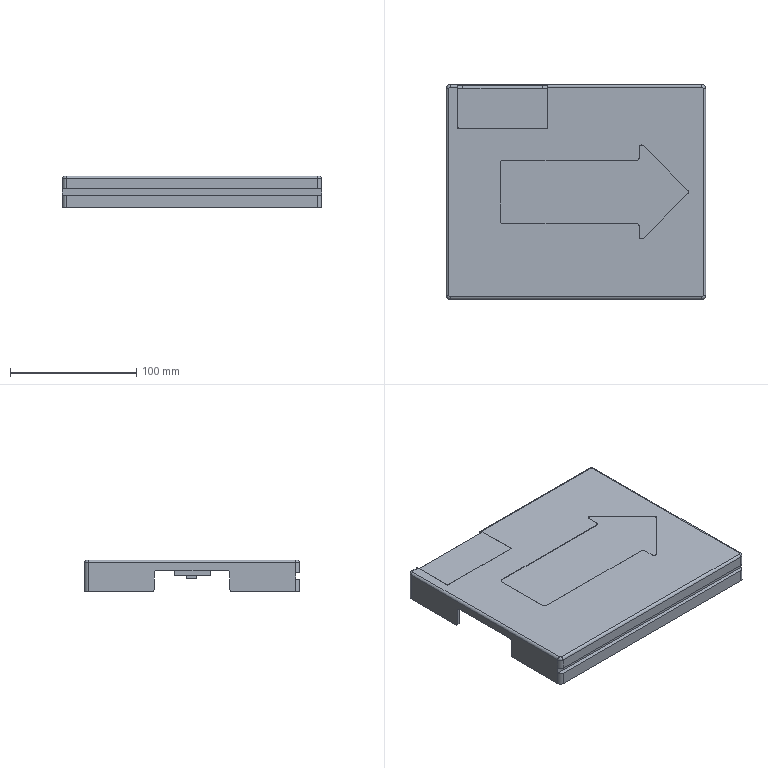NC program | NX | posted with a generic post | part box 205 x 170 x 25 mm
Lines 12675 to 13937 of 17262:
(ZLEVEL_PROFILE_1_COPY_1 , TOOL : D3R0.5)
N25306 T07 M6
N25308 G54
N25310 G17 G0 G90 X99.394 Y-30.534 B0. C0. S9500 M3
N25312 G43 Z30. H7
N25314 Z0.991
N25316 G94 G1 Z-0.009 F1000.
N25318 X99.711 Y-30.848
N25320 G3 X100.001 Y-30.925 R0.3
N25322 G1 X100.5 Y-30.789 F2500.
N25324 X102.5
N25326 X103.04 Y-30.943
N25328 X103.024 Y-30.869 Z-0.019
N25330 G3 X102.5 Y-30.709 R1.438
N25332 G1 X100.5
N25334 X99.999 Y-30.837
N25336 Y-30.78 Z-0.025
N25338 Y-30.732 Z-0.03
N25340 X100.5 Y-30.613
N25342 X102.5
N25344 X103.001 Y-30.741
N25346 Y-30.69 Z-0.038
N25348 Y-30.671 Z-0.046
N25350 G3 X102.5 Y-30.541 R1.095
N25352 G1 X100.5
N25354 X99.981 Y-30.655
N25356 Y-30.603 Z-0.055
N25358 Y-30.541 Z-0.065
N25360 X100.5 Y-30.435
N25362 X102.5
N25364 G2 X103. Y-30.565 R1.064
N25366 G1 X102.999 Y-30.47 Z-0.086
N25368 X102.5 Y-30.348
N25370 X100.5
N25372 X99.997 Y-30.447
N25374 Y-30.42 Z-0.099
N25376 X99.996 Y-30.365 Z-0.112
N25378 X100.5 Y-30.259
N25380 X102.5
N25382 X102.999 Y-30.387
N25384 Y-30.328 Z-0.127
N25386 Y-30.291 Z-0.142
N25388 G3 X102.5 Y-30.17 R1.236
N25390 G1 X100.5
N25392 X99.996 Y-30.272
N25394 Y-30.24 Z-0.158
N25396 X99.997 Y-30.185 Z-0.175
N25398 X100.5 Y-30.082
N25400 X102.5
N25402 X102.999 Y-30.199
N25404 X103. Y-30.146 Z-0.193
N25406 X103.001 Y-30.104 Z-0.211
N25408 X102.5 Y-29.994
N25410 X100.5
N25412 X99.997 Y-30.093
N25414 X99.998 Y-30.058 Z-0.231
N25416 X99.999 Y-30.004 Z-0.251
N25418 X100.5 Y-29.908
N25420 X102.5
N25422 X103.001 Y-30.006
N25424 Y-29.968 Z-0.273
N25426 X103.002 Y-29.918 Z-0.295
N25428 X102.5 Y-29.822
N25430 X100.5
N25432 X99.998 Y-29.913
N25434 Y-29.883 Z-0.318
N25436 Y-29.824 Z-0.342
N25438 G2 X100.5 Y-29.738 R3.15
N25440 G1 X102.5
N25442 X102.552 Y-29.741
N25444 X103.002 Y-29.829
N25446 Y-29.792 Z-0.367
N25448 Y-29.738 Z-0.392
N25450 X102.5 Y-29.655
N25452 X100.5
N25454 X99.999 Y-29.736
N25456 Y-29.696 Z-0.419
N25458 Y-29.65 Z-0.446
N25460 X100.5 Y-29.574
N25462 X102.5
N25464 X103.003 Y-29.643
N25466 Y-29.61 Z-0.475
N25468 X103.002 Y-29.566 Z-0.504
N25470 X102.5 Y-29.495
N25472 X100.5
N25474 X99.999 Y-29.569
N25476 Y-29.533 Z-0.534
N25478 X100. Y-29.491 Z-0.564
N25480 X100.5 Y-29.418
N25482 X102.5
N25484 G2 X103. Y-29.496 R37.012
N25486 G1 Y-29.457 Z-0.596
N25488 Y-29.419 Z-0.628
N25490 X102.5 Y-29.343
N25492 X100.5
N25494 X100. Y-29.417
N25496 Y-29.378 Z-0.661
N25498 Y-29.339 Z-0.694
N25500 G3 X100.5 Y-29.271 R1996.585
N25502 G1 X102.5
N25504 X103. Y-29.338
N25506 Y-29.299 Z-0.729
N25508 Y-29.26 Z-0.764
N25510 X102.944
N25512 X102.5 Y-29.201
N25514 X100.5
N25516 G2 X100. Y-29.262 R13.454
N25518 G1 Y-29.228 Z-0.8
N25520 Y-29.201 Z-0.837
N25522 G3 X100.5 Y-29.134 R9.112
N25524 G1 X102.5
N25526 G3 X103. Y-29.199 R5.937
N25528 G1 Y-29.164 Z-0.874
N25530 Y-29.136 Z-0.912
N25532 G2 X102.5 Y-29.069 R5.444
N25534 G1 X100.5
N25536 G3 X100.103 Y-29.135 R1.782
N25538 G1 X100. Y-29.138
N25540 Y-29.101 Z-0.951
N25542 Y-29.073 Z-0.99
N25544 G3 X100.255 Y-29.031 R0.597
N25546 G1 X100.5 Y-29.008
N25548 X102.5
N25550 G2 X102.895 Y-29.069 R1.306
N25552 G1 X103. Y-29.07
N25554 Y-29.037 Z-1.03
N25556 X103.001 Y-29.001 Z-1.07
N25558 X102.5 Y-28.95
N25560 X100.5
N25562 X100.348 Y-28.96
N25564 G2 X100. Y-29.007 R1.243
N25566 G1 Y-28.975 Z-1.111
N25568 Y-28.948 Z-1.152
N25570 G3 X100.348 Y-28.903 R1.222
N25572 G1 X100.5 Y-28.894
N25574 X102.5
N25576 X103.001 Y-28.943
N25578 Y-28.921 Z-1.195
N25580 Y-28.893 Z-1.237
N25582 X102.5 Y-28.842
N25584 X100.5
N25586 X100.348 Y-28.854
N25588 G2 X100. Y-28.899 R1.238
N25590 G1 Y-28.873 Z-1.281
N25592 Y-28.853 Z-1.324
N25594 G3 X100.348 Y-28.803 R1.115
N25596 G1 X100.5 Y-28.794
N25598 X102.5
N25600 X103.001 Y-28.847
N25602 Y-28.826 Z-1.369
N25604 X103. Y-28.8 Z-1.413
N25606 X102.5 Y-28.749
N25608 X100.5
N25610 G3 X100.111 Y-28.799 R2.259
N25612 G1 X100.056 Y-28.817
N25614 X100. Y-28.805
N25616 Y-28.778 Z-1.458
N25618 Y-28.758 Z-1.504
N25620 X100.103 Y-28.755
N25622 G2 X100.5 Y-28.707 R3.348
N25624 G1 X102.5
N25626 G3 X103.001 Y-28.754 R4.196
N25628 G1 Y-28.738 Z-1.55
N25630 Y-28.714 Z-1.596
N25632 G2 X102.5 Y-28.669 R6.317
N25634 G1 X100.5
N25636 G3 X100.103 Y-28.715 R2.341
N25638 G1 X99.999 Y-28.718
N25640 Y-28.701 Z-1.643
N25642 Y-28.688 Z-1.69
N25644 X100.103 Y-28.686
N25646 G2 X100.5 Y-28.635 R1.961
N25648 G1 X102.5
N25650 X103.003 Y-28.683
N25652 Y-28.671 Z-1.737
N25654 Y-28.654 Z-1.785
N25656 X102.5 Y-28.604
N25658 X100.5
N25660 G3 X100.103 Y-28.656 R1.723
N25662 G1 X99.999 Y-28.659
N25664 Y-28.641 Z-1.833
N25666 Y-28.629 Z-1.881
N25668 X100.103 Y-28.626
N25670 G2 X100.5 Y-28.578 R2.479
N25672 G1 X102.5
N25674 X103.003 Y-28.624
N25676 Y-28.615 Z-1.93
N25678 Y-28.599 Z-1.978
N25680 X102.5 Y-28.555
N25682 X100.5
N25684 G3 X100.103 Y-28.6 R3.094
N25686 G1 X99.999 Y-28.602
N25688 X99.998 Y-28.589 Z-2.028
N25690 Y-28.585 Z-2.077
N25692 X100.103 Y-28.58
N25694 G2 X100.5 Y-28.536 R2.159
N25696 G1 X102.5
N25698 G2 X103.002 Y-28.583 R25.83
N25700 G1 Y-28.572 Z-2.126
N25702 X103.001 Y-28.568 Z-2.176
N25704 X102.5 Y-28.521
N25706 X100.5
N25708 X100.232 Y-28.546
N25710 G2 X99.999 Y-28.571 R0.934
N25712 G1 Y-28.564 Z-2.225
N25714 Y-28.56 Z-2.275
N25716 X100.16 Y-28.546
N25718 G2 X100.5 Y-28.51 R2.032
N25720 G1 X102.5
N25722 G3 X103. Y-28.553 R6.443
N25724 G1 Y-28.546 Z-2.325
N25726 Y-28.539 Z-2.375
N25728 G2 X102.5 Y-28.503 R5.294
N25730 G1 X100.5
N25732 G3 X100. Y-28.549 R57.724
N25734 G1 Y-28.54 Z-2.475
N25736 X100.5 Y-28.5
N25738 X102.5
N25740 G3 X103. Y-28.53 R3.832
N25742 G1 Y-28.529 Z-2.575
N25744 G2 X102.5 Y-28.5 R3.541
N25746 G1 X100.5
N25748 X100. Y-28.536
N25750 Y-28.534 Z-2.675
N25752 X100.5 Y-28.5
N25754 X100.616
N25756 X101.802
N25758 X101.863
N25760 X102.408
N25762 X102.5
N25764 G3 X103. Y-28.527 R3.401
N25766 G1 Y-28.525 Z-2.775
N25768 G2 X102.5 Y-28.5 R3.458
N25770 G1 X102.408
N25772 X101.863
N25774 X101.802
N25776 X101.756
N25778 X100.616
N25780 X100.5
N25782 X100. Y-28.532
N25784 Y-28.531 Z-2.875
N25786 G2 X100.5 Y-28.5 R8.281
N25788 G1 X100.616
N25790 X101.802
N25792 X101.863
N25794 X102.408
N25796 X102.5
N25798 G3 X103. Y-28.524 R3.678
N25800 G1 Y-28.522 Z-2.975
N25802 G2 X102.5 Y-28.5 R3.929
N25804 G1 X102.408
N25806 X101.863
N25808 X101.802
N25810 X101.756
N25812 X100.616
N25814 X100.5
N25816 G3 X100. Y-28.529 R7.641
N25818 G1 Y-28.527 Z-3.075
N25820 G2 X100.5 Y-28.5 R202.736
N25822 G1 X100.616
N25824 X101.802
N25826 X101.863
N25828 X102.408
N25830 X102.5
N25832 G3 X103. Y-28.521 R4.217
N25834 G1 Y-28.519 Z-3.175
N25836 G2 X102.5 Y-28.5 R4.551
N25838 G1 X102.408
N25840 X101.863
N25842 X101.802
N25844 X101.756
N25846 X100.616
N25848 X100.5
N25850 X100. Y-28.525
N25852 Y-28.523 Z-3.275
N25854 X100.5 Y-28.5
N25856 X100.616
N25858 X101.802
N25860 X101.863
N25862 X102.408
N25864 X102.5
N25866 G3 X103. Y-28.518 R4.942
N25868 G1 Y-28.516 Z-3.375
N25870 G2 X102.5 Y-28.5 R5.408
N25872 G1 X102.408
N25874 X101.863
N25876 X101.802
N25878 X101.756
N25880 X100.616
N25882 X100.5
N25884 X100. Y-28.522
N25886 Y-28.52 Z-3.475
N25888 X100.5 Y-28.5
N25890 X100.616
N25892 X101.802
N25894 X101.863
N25896 X102.408
N25898 X102.5
N25900 G3 X103. Y-28.515 R5.363
N25902 G1 Y-28.513 Z-3.575
N25904 G2 X102.5 Y-28.5 R5.209
N25906 G1 X102.408
N25908 X101.863
N25910 X101.802
N25912 X101.756
N25914 X100.616
N25916 X100.5
N25918 X100. Y-28.519
N25920 Y-28.518 Z-3.675
N25922 X100.5 Y-28.5
N25924 X100.616
N25926 X101.802
N25928 X101.863
N25930 X102.408
N25932 X102.5
N25934 G3 X103. Y-28.512 R5.064
N25936 G1 Y-28.511 Z-3.775
N25938 G2 X102.5 Y-28.5 R4.927
N25940 G1 X102.408
N25942 X101.863
N25944 X101.802
N25946 X101.756
N25948 X100.616
N25950 X100.5
N25952 X100. Y-28.517
N25954 Y-28.516 Z-3.875
N25956 X100.5 Y-28.5
N25958 X100.616
N25960 X101.802
N25962 X101.863
N25964 X102.408
N25966 X102.5
N25968 G3 X103. Y-28.51 R4.797
N25970 G1 Y-28.508 Z-3.975
N25972 G2 X102.5 Y-28.5 R4.674
N25974 G1 X102.408
N25976 X101.863
N25978 X101.802
N25980 X101.756
N25982 X100.616
N25984 X100.5
N25986 X100. Y-28.515
N25988 Y-28.514 Z-4.075
N25990 X100.5 Y-28.5
N25992 X100.616
N25994 X101.802
N25996 X101.863
N25998 X102.408
N26000 X102.5
N26002 G3 X103. Y-28.507 R4.558
N26004 G1 Y-28.506 Z-4.175
N26006 G2 X102.5 Y-28.5 R4.446
N26008 G1 X102.408
N26010 X101.863
N26012 X101.802
N26014 X101.756
N26016 X100.616
N26018 X100.5
N26020 X100. Y-28.512
N26022 Y-28.511 Z-4.275
N26024 X100.5 Y-28.5
N26026 X100.616
N26028 X101.802
N26030 X101.863
N26032 X102.408
N26034 X102.5
N26036 G3 X103. Y-28.505 R4.385
N26038 G1 Z-4.375
N26040 G2 X102.5 Y-28.5 R4.589
N26042 G1 X102.408
N26044 X101.863
N26046 X101.802
N26048 X101.756
N26050 X100.616
N26052 X100.5
N26054 X100. Y-28.51
N26056 Z-4.475
N26058 X100.5 Y-28.5
N26060 X100.616
N26062 X101.802
N26064 X101.863
N26066 X102.408
N26068 X102.5
N26070 G3 X103. Y-28.504 R4.812
N26072 G1 Z-4.575
N26074 G2 X102.5 Y-28.5 R20.562
N26076 G1 X102.408
N26078 X101.863
N26080 X101.802
N26082 X101.756
N26084 X100.616
N26086 X100.5
N26088 X100. Y-28.51
N26090 Y-28.509 Z-4.675
N26092 X100.5 Y-28.5
N26094 X100.616
N26096 X101.802
N26098 X101.863
N26100 X102.408
N26102 X102.5
N26104 G3 X103. Y-28.503 R21.332
N26106 G1 Z-4.775
N26108 G2 X102.5 Y-28.5 R22.858
N26110 G1 X102.408
N26112 X101.863
N26114 X101.802
N26116 X101.756
N26118 X100.616
N26120 X100.5
N26122 X100. Y-28.509
N26124 Y-28.508 Z-4.875
N26126 X100.5 Y-28.5
N26128 X100.616
N26130 X101.802
N26132 X101.863
N26134 X102.408
N26136 X102.5
N26138 G3 X103. Y-28.503 R25.34
N26140 G1 Z-4.975
N26142 X102.5 Y-28.5
N26144 X102.408
N26146 X101.863
N26148 X101.802
N26150 X101.756
N26152 X100.616
N26154 X100.5
N26156 X100. Y-28.508
N26158 Y-28.507 Z-5.075
N26160 X100.5 Y-28.5
N26162 X100.616
N26164 X101.802
N26166 X101.863
N26168 X102.408
N26170 X102.5
N26172 X103. Y-28.503
N26174 Z-5.175
N26176 X102.5 Y-28.5
N26178 X102.408
N26180 X101.863
N26182 X101.802
N26184 X101.756
N26186 X100.616
N26188 X100.5
N26190 X100. Y-28.507
N26192 Z-5.275
N26194 X100.5 Y-28.5
N26196 X100.616
N26198 X101.802
N26200 X101.863
N26202 X102.408
N26204 X102.5
N26206 X103. Y-28.502
N26208 Z-5.375
N26210 X102.5 Y-28.5
N26212 X102.408
N26214 X101.863
N26216 X101.802
N26218 X101.756
N26220 X100.616
N26222 X100.5
N26224 X100. Y-28.506
N26226 Z-5.475
N26228 X100.5 Y-28.5
N26230 X100.616
N26232 X101.802
N26234 X101.863
N26236 X102.408
N26238 X102.5
N26240 X103. Y-28.502
N26242 Z-5.575
N26244 X102.5 Y-28.5
N26246 X102.408
N26248 X101.863
N26250 X101.802
N26252 X101.756
N26254 X100.616
N26256 X100.5
N26258 X100. Y-28.505
N26260 Z-5.675
N26262 X100.5 Y-28.5
N26264 X100.616
N26266 X101.802
N26268 X101.863
N26270 X102.408
N26272 X102.5
N26274 X102.552
N26276 X103. Y-28.502
N26278 Z-5.775
N26280 X102.5 Y-28.5
N26282 X102.408
N26284 X101.863
N26286 X101.802
N26288 X101.756
N26290 X100.616
N26292 X100.5
N26294 X100. Y-28.505
N26296 X100.001 Y-28.504 Z-5.875
N26298 X100.5 Y-28.5
N26300 X100.616
N26302 X101.802
N26304 X101.863
N26306 X102.408
N26308 X102.5
N26310 X103. Y-28.502
N26312 Y-28.501 Z-5.975
N26314 X102.5 Y-28.5
N26316 X102.408
N26318 X101.863
N26320 X101.802
N26322 X101.756
N26324 X100.616
N26326 X100.5
N26328 X100.001 Y-28.504
N26330 Y-28.503 Z-6.075
N26332 X100.5 Y-28.5
N26334 X100.616
N26336 X101.802
N26338 X101.863
N26340 X102.408
N26342 X102.5
N26344 X103. Y-28.501
N26346 Z-6.175
N26348 X102.5 Y-28.5
N26350 X102.408
N26352 X101.863
N26354 X101.802
N26356 X101.756
N26358 X100.616
N26360 X100.5
N26362 X100.001 Y-28.503
N26364 Z-6.275
N26366 X100.5 Y-28.5
N26368 X100.616
N26370 X101.802
N26372 X101.863
N26374 X102.408
N26376 X102.5
N26378 X103. Y-28.501
N26380 Z-6.375
N26382 X102.5 Y-28.5
N26384 X102.408
N26386 X101.863
N26388 X101.802
N26390 X101.756
N26392 X100.616
N26394 X100.5
N26396 X100.001 Y-28.503
N26398 Z-6.475
N26400 X100.5 Y-28.5
N26402 X100.616
N26404 X101.802
N26406 X101.863
N26408 X102.408
N26410 X102.5
N26412 X103. Y-28.501
N26414 Z-6.575
N26416 X102.5 Y-28.5
N26418 X102.408
N26420 X101.863
N26422 X101.802
N26424 X101.756
N26426 X100.616
N26428 X100.5
N26430 X100.001 Y-28.503
N26432 Z-6.675
N26434 X100.5 Y-28.5
N26436 X100.616
N26438 X101.802
N26440 X101.863
N26442 X102.408
N26444 X102.5
N26446 X103. Y-28.501
N26448 Z-6.775
N26450 X102.5 Y-28.5
N26452 X102.408
N26454 X101.863
N26456 X101.802
N26458 X101.756
N26460 X100.616
N26462 X100.5
N26464 X100.001 Y-28.503
N26466 Z-6.875
N26468 X100.5 Y-28.5
N26470 X100.616
N26472 X101.802
N26474 X101.863
N26476 X102.408
N26478 X102.5
N26480 X103. Y-28.501
N26482 Z-6.975
N26484 X102.5 Y-28.5
N26486 X102.408
N26488 X101.863
N26490 X101.802
N26492 X101.756
N26494 X100.616
N26496 X100.5
N26498 X100.001 Y-28.503
N26500 Z-7.075
N26502 X100.5 Y-28.5
N26504 X100.616
N26506 X101.802
N26508 X101.863
N26510 X102.408
N26512 X102.5
N26514 X103. Y-28.501
N26516 Z-7.175
N26518 X102.5 Y-28.5
N26520 X102.408
N26522 X101.863
N26524 X101.802
N26526 X101.756
N26528 X100.616
N26530 X100.5
N26532 X100.001 Y-28.503
N26534 Z-7.275
N26536 X100.5 Y-28.5
N26538 X100.616
N26540 X101.802
N26542 X101.863
N26544 X102.408
N26546 X102.5
N26548 X103. Y-28.501
N26550 Z-7.375
N26552 X102.5 Y-28.5
N26554 X102.408
N26556 X101.863
N26558 X101.802
N26560 X101.756
N26562 X100.616
N26564 X100.5
N26566 X100.001 Y-28.503
N26568 Z-7.475
N26570 X100.5 Y-28.5
N26572 X100.616
N26574 X101.802
N26576 X101.863
N26578 X102.408
N26580 X102.5
N26582 X103. Y-28.501
N26584 Z-7.575
N26586 X102.5 Y-28.5
N26588 X102.408
N26590 X101.863
N26592 X101.802
N26594 X101.756
N26596 X100.616
N26598 X100.5
N26600 X100.001 Y-28.503
N26602 Z-7.675
N26604 X100.5 Y-28.5
N26606 X100.616
N26608 X101.802
N26610 X101.863
N26612 X102.408
N26614 X102.5
N26616 X103. Y-28.501
N26618 Z-7.775
N26620 X102.5 Y-28.5
N26622 X102.408
N26624 X101.863
N26626 X101.802
N26628 X101.756
N26630 X100.616
N26632 X100.5
N26634 X100.001 Y-28.503
N26636 X100.002 Z-7.875
N26638 X100.5 Y-28.5
N26640 X100.616
N26642 X101.802
N26644 X101.863
N26646 X102.408
N26648 X102.5
N26650 X103. Y-28.501
N26652 Z-7.975
N26654 X102.5 Y-28.5
N26656 X102.408
N26658 X101.863
N26660 X101.802
N26662 X101.756
N26664 X100.616
N26666 X100.5
N26668 X100.002 Y-28.503
N26670 Z-8.075
N26672 X100.5 Y-28.5
N26674 X100.616
N26676 X101.802
N26678 X101.863
N26680 X102.408
N26682 X102.5
N26684 X103.
N26686 Z-8.175
N26688 X102.5
N26690 X102.408
N26692 X101.863
N26694 X101.802
N26696 X101.756
N26698 X100.616
N26700 X100.5
N26702 X100.002 Y-28.503
N26704 Z-8.275
N26706 X100.5 Y-28.5
N26708 X100.616
N26710 X101.802
N26712 X101.863
N26714 X102.408
N26716 X102.5
N26718 X103.
N26720 Z-8.375
N26722 X102.5
N26724 X102.408
N26726 X101.863
N26728 X101.802
N26730 X101.756
N26732 X100.616
N26734 X100.5
N26736 X100.002 Y-28.503
N26738 Z-8.475
N26740 X100.5 Y-28.5
N26742 X100.616
N26744 X101.802
N26746 X101.863
N26748 X102.408
N26750 X102.5
N26752 X103.
N26754 Z-8.575
N26756 X102.5
N26758 X102.408
N26760 X101.863
N26762 X101.802
N26764 X101.756
N26766 X100.616
N26768 X100.5
N26770 X100.002 Y-28.503
N26772 Z-8.675
N26774 X100.5 Y-28.5
N26776 X100.616
N26778 X101.802
N26780 X101.863
N26782 X102.408
N26784 X102.5
N26786 X103.
N26788 Z-8.775
N26790 X102.5
N26792 X102.408
N26794 X101.863
N26796 X101.802
N26798 X101.756
N26800 X100.616
N26802 X100.5
N26804 X100.002 Y-28.503
N26806 Z-8.875
N26808 X100.5 Y-28.5
N26810 X100.616
N26812 X101.802
N26814 X101.863
N26816 X102.408
N26818 X102.5
N26820 X103.
N26822 Z-8.975
N26824 X102.5
N26826 X102.408
N26828 X101.863
N26830 X101.802
N26832 X101.756
N26834 X100.616
N26836 X100.5
N26838 X100.002 Y-28.503
N26840 Z-9.075
N26842 X100.5 Y-28.5
N26844 X100.616
N26846 X101.802
N26848 X101.863
N26850 X102.408
N26852 X102.5
N26854 X103.
N26856 Z-9.175
N26858 X102.5
N26860 X102.408
N26862 X101.863
N26864 X101.802
N26866 X101.756
N26868 X100.616
N26870 X100.5
N26872 X100.002 Y-28.503
N26874 Z-9.275
N26876 X100.5 Y-28.5
N26878 X100.616
N26880 X101.802
N26882 X101.863
N26884 X102.408
N26886 X102.5
N26888 X103.
N26890 Z-9.375
N26892 X102.5
N26894 X102.408
N26896 X101.863
N26898 X101.802
N26900 X101.756
N26902 X100.616
N26904 X100.5
N26906 X100.002 Y-28.503
N26908 Z-9.475
N26910 X100.5 Y-28.5
N26912 X100.616
N26914 X101.802
N26916 X101.863
N26918 X102.408
N26920 X102.5
N26922 X103.
N26924 Z-9.575
N26926 X102.5
N26928 X102.408
N26930 X101.863
N26932 X101.802
N26934 X101.756
N26936 X100.616
N26938 X100.5
N26940 X100.002 Y-28.502
N26942 Z-9.675
N26944 X100.5 Y-28.5
N26946 X100.616
N26948 X101.802
N26950 X101.863
N26952 X102.408
N26954 X102.5
N26956 X103.
N26958 Z-9.775
N26960 X102.5
N26962 X102.408
N26964 X101.863
N26966 X101.802
N26968 X101.756
N26970 X100.616
N26972 X100.5
N26974 X100.002 Y-28.502
N26976 Z-9.875
N26978 X100.5 Y-28.5
N26980 X100.616
N26982 X101.802
N26984 X101.863
N26986 X102.408
N26988 X102.5
N26990 X103.
N26992 Z-9.975
N26994 X102.5
N26996 X102.408
N26998 X101.863
N27000 X101.802
N27002 X101.756
N27004 X100.616
N27006 X100.5
N27008 X100.002 Y-28.502
N27010 Z-10.075
N27012 X100.5 Y-28.5
N27014 X100.616
N27016 X101.802
N27018 X101.863
N27020 X102.408
N27022 X102.5
N27024 X103.
N27026 Z-10.175
N27028 X102.5
N27030 X102.408
N27032 X101.863
N27034 X101.802
N27036 X101.756
N27038 X100.616
N27040 X100.5
N27042 X100.002 Y-28.502
N27044 Z-10.275
N27046 X100.5 Y-28.5
N27048 X100.616
N27050 X101.802
N27052 X101.863
N27054 X102.408
N27056 X102.5
N27058 X103.
N27060 Y-28.499 Z-10.375
N27062 X102.5 Y-28.5
N27064 X102.408
N27066 X101.863
N27068 X101.802
N27070 X101.756
N27072 X100.616
N27074 X100.5
N27076 X100.002 Y-28.502
N27078 Z-10.475
N27080 X100.5 Y-28.5
N27082 X100.616
N27084 X101.802
N27086 X101.863
N27088 X102.408
N27090 X102.5
N27092 X103. Y-28.499
N27094 Z-10.575
N27096 X102.5 Y-28.5
N27098 X102.408
N27100 X101.863
N27102 X101.802
N27104 X101.756
N27106 X100.616
N27108 X100.5
N27110 X100.002 Y-28.502
N27112 Z-10.675
N27114 X100.5 Y-28.5
N27116 X100.616
N27118 X101.802
N27120 X101.863
N27122 X102.408
N27124 X102.5
N27126 X103. Y-28.499
N27128 Z-10.775
N27130 X102.5 Y-28.5
N27132 X102.408
N27134 X101.863
N27136 X101.802
N27138 X101.756
N27140 X100.616
N27142 X100.5
N27144 X100.002 Y-28.502
N27146 Z-10.875
N27148 X100.5 Y-28.5
N27150 X100.616
N27152 X101.802
N27154 X101.863
N27156 X102.408
N27158 X102.5
N27160 X103. Y-28.499
N27162 Z-10.975
N27164 X102.5 Y-28.5
N27166 X102.408
N27168 X101.863
N27170 X101.802
N27172 X101.756
N27174 X100.616
N27176 X100.5
N27178 X100.002 Y-28.502
N27180 Z-11.075
N27182 X100.5 Y-28.5
N27184 X100.616
N27186 X101.802
N27188 X101.863
N27190 X102.408
N27192 X102.5
N27194 X103. Y-28.499
N27196 Z-11.175
N27198 X102.5 Y-28.5
N27200 X102.408
N27202 X101.863
N27204 X101.802
N27206 X101.756
N27208 X100.616
N27210 X100.5
N27212 X100.002 Y-28.502
N27214 Z-11.275
N27216 X100.5 Y-28.5
N27218 X100.616
N27220 X101.802
N27222 X101.863
N27224 X102.408
N27226 X102.5
N27228 X103. Y-28.499
N27230 Z-11.375
N27232 X102.5 Y-28.5
N27234 X102.408
N27236 X101.863
N27238 X101.802
N27240 X101.756
N27242 X100.616
N27244 X100.5
N27246 X100.002 Y-28.502
N27248 Z-11.475
N27250 X100.5 Y-28.5
N27252 X100.616
N27254 X101.802
N27256 X101.863
N27258 X102.408
N27260 X102.5
N27262 X103. Y-28.499
N27264 Z-11.575
N27266 X102.5 Y-28.5
N27268 X102.408
N27270 X101.863
N27272 X101.802
N27274 X101.756
N27276 X100.616
N27278 X100.5
N27280 X100.003 Y-28.502
N27282 Z-11.675
N27284 X100.5 Y-28.5
N27286 X100.616
N27288 X101.802
N27290 X101.863
N27292 X102.408
N27294 X102.5
N27296 X103. Y-28.499
N27298 Z-11.775
N27300 X102.5 Y-28.5
N27302 X102.408
N27304 X101.863
N27306 X101.802
N27308 X101.756
N27310 X100.616
N27312 X100.5
N27314 X100.003 Y-28.502
N27316 Z-11.875
N27318 X100.5 Y-28.5
N27320 X100.616
N27322 X101.802
N27324 X101.863
N27326 X102.408
N27328 X102.5
N27330 X103. Y-28.499
N27332 Z-11.975
N27334 X102.5 Y-28.5
N27336 X102.408
N27338 X101.863
N27340 X101.802
N27342 X101.756
N27344 X100.616
N27346 X100.5
N27348 X100.003 Y-28.502
N27350 Z-12.075
N27352 X100.5 Y-28.5
N27354 X100.616
N27356 X101.802
N27358 X101.863
N27360 X102.408
N27362 X102.5
N27364 X103. Y-28.499
N27366 Z-12.175
N27368 X102.5 Y-28.5
N27370 X102.408
N27372 X101.863
N27374 X101.802
N27376 X101.756
N27378 X100.616
N27380 X100.5
N27382 X100.003 Y-28.502
N27384 Z-12.275
N27386 X100.5 Y-28.5
N27388 X100.616
N27390 X101.802
N27392 X101.863
N27394 X102.408
N27396 X102.5
N27398 X103. Y-28.499
N27400 Z-12.375
N27402 X102.5 Y-28.5
N27404 X102.408
N27406 X101.863
N27408 X101.802
N27410 X101.756
N27412 X100.616
N27414 X100.5
N27416 X100.003 Y-28.501
N27418 Z-12.475
N27420 X100.5 Y-28.5
N27422 X100.616
N27424 X101.802
N27426 X101.863
N27428 X102.408
N27430 X102.5
N27432 X103. Y-28.498
N27434 Z-12.575
N27436 X102.5 Y-28.5
N27438 X102.408
N27440 X101.863
N27442 X101.802
N27444 X101.756
N27446 X100.616
N27448 X100.5
N27450 X100.003 Y-28.501
N27452 Z-12.675
N27454 X100.5 Y-28.5
N27456 X100.616
N27458 X101.802
N27460 X101.863
N27462 X102.408
N27464 X102.5
N27466 X103. Y-28.498
N27468 Z-12.775
N27470 X102.5 Y-28.5
N27472 X102.408
N27474 X101.863
N27476 X101.802
N27478 X101.756
N27480 X100.616
N27482 X100.5
N27484 X100.003 Y-28.501
N27486 Z-12.875
N27488 X100.5 Y-28.5
N27490 X100.616
N27492 X101.802
N27494 X101.863
N27496 X102.408
N27498 X102.5
N27500 X103. Y-28.498
N27502 X103.001 Z-12.975
N27504 X102.5 Y-28.5
N27506 X102.408
N27508 X101.863
N27510 X101.802
N27512 X101.756
N27514 X100.616
N27516 X100.5
N27518 X100.003 Y-28.501
N27520 Z-13.075
N27522 X100.5 Y-28.5
N27524 X100.616
N27526 X101.802
N27528 X101.863
N27530 X102.408
N27532 X102.5
N27534 X103.001 Y-28.497
N27536 Z-13.175
N27538 X102.5 Y-28.5
N27540 X102.408
N27542 X101.863
N27544 X101.802
N27546 X101.756
N27548 X100.616
N27550 X100.5
N27552 X100.003 Y-28.501
N27554 X100.004 Y-28.5 Z-13.275
N27556 X100.5
N27558 X100.616
N27560 X101.802
N27562 X101.863
N27564 X102.408
N27566 X102.5
N27568 X103.001 Y-28.496
N27570 Z-13.375
N27572 X102.5 Y-28.5
N27574 X102.408
N27576 X101.863
N27578 X101.802
N27580 X101.756
N27582 X100.616
N27584 X100.5
N27586 X100.004
N27588 Z-13.475
N27590 X100.5
N27592 X100.616
N27594 X101.802
N27596 X101.863
N27598 X102.408
N27600 X102.5
N27602 X103.001 Y-28.496
N27604 Y-28.495 Z-13.575
N27606 X102.5 Y-28.5
N27608 X102.408
N27610 X101.863
N27612 X101.802
N27614 X101.756
N27616 X100.616
N27618 X100.5
N27620 X100.103 Y-28.497
N27622 X100.004 Y-28.5
N27624 X100.005 Z-13.675
N27626 X100.103 Y-28.497
N27628 X100.5 Y-28.5
N27630 X100.616
N27632 X101.802
N27634 X101.863
N27636 X102.408
N27638 X102.5
N27640 X103.001 Y-28.495
N27642 Y-28.494 Z-13.775
N27644 X102.5 Y-28.5
N27646 X102.408
N27648 X101.863
N27650 X101.802
N27652 X101.756
N27654 X100.616
N27656 X100.5
N27658 X100.418 Y-28.497
N27660 X100.004 Y-28.499
N27662 Y-28.497 Z-13.875
N27664 X100.103 Y-28.495
N27666 X100.514 Y-28.497
N27668 X100.552 Y-28.5
N27670 X100.616
N27672 X101.802
N27674 X101.863
N27676 X102.408
N27678 X102.5
N27680 X103.001 Y-28.492
N27682 X103.002 Y-28.491 Z-13.975
N27684 X102.5 Y-28.5
N27686 X102.408
N27688 X101.863
N27690 X101.802
N27692 X101.756
N27694 X100.616
N27696 X100.553
N27698 X100.534 Y-28.497
N27700 X100.103 Y-28.493
N27702 X100.004 Y-28.496
N27704 Y-28.495 Z-14.075
N27706 X100.103 Y-28.492
N27708 X100.553 Y-28.5
N27710 X100.616
N27712 X101.802
N27714 X101.863
N27716 X102.408
N27718 X102.5
N27720 X103.002 Y-28.489
N27722 X103.003 Y-28.487 Z-14.175
N27724 X102.5 Y-28.5
N27726 X102.408
N27728 X101.863
N27730 X101.802
N27732 X101.756
N27734 X100.616
N27736 X100.554
N27738 X100.103 Y-28.491
N27740 X100.004 Y-28.493
N27742 Y-28.492 Z-14.275
N27744 G2 X100.557 Y-28.5 R5.056
N27746 G1 X100.616
N27748 X101.802
N27750 X101.863
N27752 X102.408
N27754 X102.5
N27756 X103.003 Y-28.485
N27758 X103.004 Y-28.483 Z-14.375
N27760 X102.5 Y-28.5
N27762 X102.408
N27764 X101.863
N27766 X101.802
N27768 X101.756
N27770 X100.616
N27772 X100.557
N27774 G3 X100.004 Y-28.491 R4.58
N27776 G1 Y-28.489 Z-14.475
N27778 G2 X100.558 Y-28.5 R4.188
N27780 G1 X100.616
N27782 X101.802
N27784 X101.863
N27786 X102.408
N27788 X102.5
N27790 X103.004 Y-28.481
N27792 X103.005 Y-28.479 Z-14.575
N27794 X102.5 Y-28.5
N27796 X102.408
N27798 X101.863
N27800 X101.802
N27802 X101.756
N27804 X100.616
N27806 X100.558
N27808 G3 X100.004 Y-28.488 R3.859
N27810 G1 X100.005 Y-28.486 Z-14.675
N27812 G2 X100.558 Y-28.5 R3.578
N27814 G1 X100.616
N27816 X101.802
N27818 X101.863
N27820 X102.408
N27822 X102.5
N27824 X103.005 Y-28.476